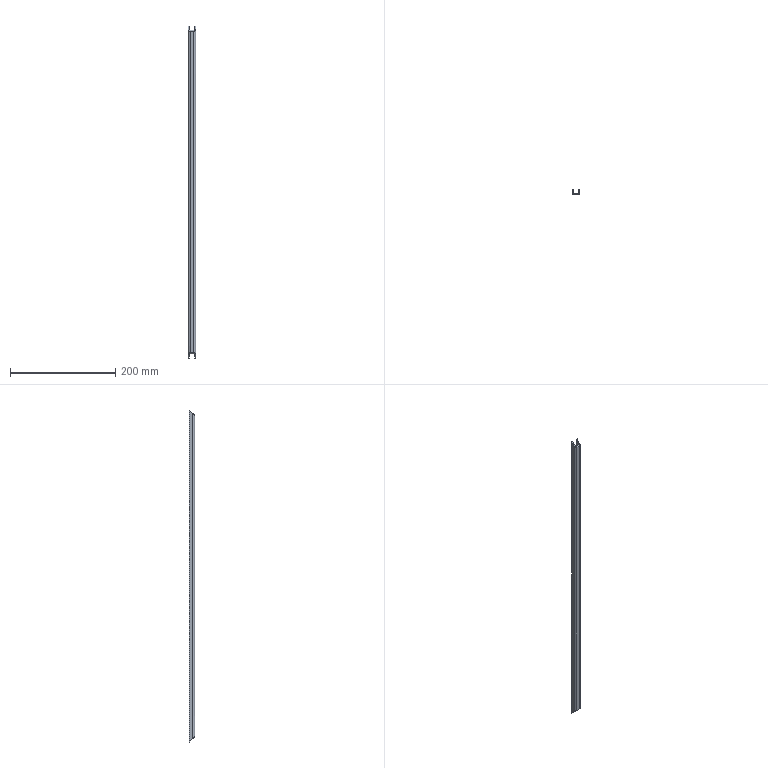Part | STEP file | 1 solid | 14 faces | box 14 x 10 x 632 mm | volume 34530 mm3 | plane 10 | cylinder 4 | commonest cylinder face diameters 3 x2 7 x2
STEP:
#1=CARTESIAN_POINT('',(0.,0.,0.));
#2=DIRECTION('',(0.,0.,1.));
#3=DIRECTION('',(1.,0.,0.));
#4=AXIS2_PLACEMENT_3D('',#1,#2,#3);
#5=CARTESIAN_POINT('',(-5.,5.,632.));
#6=VERTEX_POINT('',#5);
#7=CARTESIAN_POINT('',(-5.,5.,0.));
#8=VERTEX_POINT('',#7);
#9=CARTESIAN_POINT('',(-5.,5.,632.));
#10=DIRECTION('',(0.,0.,-1.));
#11=VECTOR('',#10,1.);
#12=LINE('',#9,#11);
#13=CARTESIAN_POINT('',(-5.,-5.,632.));
#14=DIRECTION('',(-1.,0.,0.));
#15=DIRECTION('',(0.,0.,1.));
#16=AXIS2_PLACEMENT_3D('',#13,#14,#15);
#17=PLANE('',#16);
#18=CARTESIAN_POINT('',(0.,10.));
#19=DIRECTION('',(-1.,0.));
#20=VECTOR('',#19,1.);
#21=LINE('',#18,#20);
#22=(GEOMETRIC_REPRESENTATION_CONTEXT(2)PARAMETRIC_REPRESENTATION_CONTEXT()REPRESENTATION_CONTEXT('',''));
#23=DEFINITIONAL_REPRESENTATION('',(#21),#22);
#24=PCURVE('',#17,#23);
#25=CARTESIAN_POINT('',(-7.,5.,632.));
#26=DIRECTION('',(0.,1.,0.));
#27=DIRECTION('',(0.,0.,1.));
#28=AXIS2_PLACEMENT_3D('',#25,#26,#27);
#29=PLANE('',#28);
#30=CARTESIAN_POINT('',(0.,2.));
#31=DIRECTION('',(-1.,0.));
#32=VECTOR('',#31,1.);
#33=LINE('',#30,#32);
#34=(GEOMETRIC_REPRESENTATION_CONTEXT(2)PARAMETRIC_REPRESENTATION_CONTEXT()REPRESENTATION_CONTEXT('',''));
#35=DEFINITIONAL_REPRESENTATION('',(#33),#34);
#36=PCURVE('',#29,#35);
#37=SURFACE_CURVE('',#12,(#24,#36),.PCURVE_S1.);
#38=EDGE_CURVE('',#6,#8,#37,.T.);
#39=ORIENTED_EDGE('',*,*,#38,.F.);
#40=CARTESIAN_POINT('',(-5.,-1.5,625.5));
#41=VERTEX_POINT('',#40);
#42=CARTESIAN_POINT('',(-5.,0.,627.));
#43=DIRECTION('',(0.,-0.7071,-0.7071));
#44=VECTOR('',#43,1.);
#45=LINE('',#42,#44);
#46=CARTESIAN_POINT('',(-5.,5.));
#47=DIRECTION('',(-0.7071,-0.7071));
#48=VECTOR('',#47,1.);
#49=LINE('',#46,#48);
#50=(GEOMETRIC_REPRESENTATION_CONTEXT(2)PARAMETRIC_REPRESENTATION_CONTEXT()REPRESENTATION_CONTEXT('',''));
#51=DEFINITIONAL_REPRESENTATION('',(#49),#50);
#52=PCURVE('',#17,#51);
#53=CARTESIAN_POINT('',(-63.,5.,632.));
#54=DIRECTION('',(0.,0.7071,-0.7071));
#55=DIRECTION('',(0.,0.7071,0.7071));
#56=AXIS2_PLACEMENT_3D('',#53,#54,#55);
#57=PLANE('',#56);
#58=CARTESIAN_POINT('',(-7.071,58.));
#59=DIRECTION('',(-1.,0.));
#60=VECTOR('',#59,1.);
#61=LINE('',#58,#60);
#62=(GEOMETRIC_REPRESENTATION_CONTEXT(2)PARAMETRIC_REPRESENTATION_CONTEXT()REPRESENTATION_CONTEXT('',''));
#63=DEFINITIONAL_REPRESENTATION('',(#61),#62);
#64=PCURVE('',#57,#63);
#65=SURFACE_CURVE('',#45,(#52,#64),.PCURVE_S1.);
#66=EDGE_CURVE('',#6,#41,#65,.T.);
#67=ORIENTED_EDGE('',*,*,#66,.T.);
#68=CARTESIAN_POINT('',(-5.,-1.5,6.5));
#69=VERTEX_POINT('',#68);
#70=CARTESIAN_POINT('',(-5.,-1.5,632.));
#71=DIRECTION('',(0.,0.,-1.));
#72=VECTOR('',#71,1.);
#73=LINE('',#70,#72);
#74=CARTESIAN_POINT('',(0.,3.5));
#75=DIRECTION('',(-1.,0.));
#76=VECTOR('',#75,1.);
#77=LINE('',#74,#76);
#78=(GEOMETRIC_REPRESENTATION_CONTEXT(2)PARAMETRIC_REPRESENTATION_CONTEXT()REPRESENTATION_CONTEXT('',''));
#79=DEFINITIONAL_REPRESENTATION('',(#77),#78);
#80=PCURVE('',#17,#79);
#81=CARTESIAN_POINT('',(-3.5,-1.5,632.));
#82=DIRECTION('',(0.,0.,-1.));
#83=DIRECTION('',(-1.,0.,0.));
#84=AXIS2_PLACEMENT_3D('',#81,#82,#83);
#85=CYLINDRICAL_SURFACE('',#84,1.5);
#86=CARTESIAN_POINT('',(6.283,0.));
#87=DIRECTION('',(0.,1.));
#88=VECTOR('',#87,1.);
#89=LINE('',#86,#88);
#90=(GEOMETRIC_REPRESENTATION_CONTEXT(2)PARAMETRIC_REPRESENTATION_CONTEXT()REPRESENTATION_CONTEXT('',''));
#91=DEFINITIONAL_REPRESENTATION('',(#89),#90);
#92=PCURVE('',#85,#91);
#93=SURFACE_CURVE('',#73,(#80,#92),.PCURVE_S1.);
#94=EDGE_CURVE('',#41,#69,#93,.T.);
#95=ORIENTED_EDGE('',*,*,#94,.T.);
#96=CARTESIAN_POINT('',(-5.,-316.,321.));
#97=DIRECTION('',(0.,0.7071,-0.7071));
#98=VECTOR('',#97,1.);
#99=LINE('',#96,#98);
#100=CARTESIAN_POINT('',(-311.,-311.));
#101=DIRECTION('',(-0.7071,0.7071));
#102=VECTOR('',#101,1.);
#103=LINE('',#100,#102);
#104=(GEOMETRIC_REPRESENTATION_CONTEXT(2)PARAMETRIC_REPRESENTATION_CONTEXT()REPRESENTATION_CONTEXT('',''));
#105=DEFINITIONAL_REPRESENTATION('',(#103),#104);
#106=PCURVE('',#17,#105);
#107=CARTESIAN_POINT('',(-63.,5.,0.));
#108=DIRECTION('',(0.,0.7071,0.7071));
#109=DIRECTION('',(0.,-0.7071,0.7071));
#110=AXIS2_PLACEMENT_3D('',#107,#108,#109);
#111=PLANE('',#110);
#112=CARTESIAN_POINT('',(453.963,58.));
#113=DIRECTION('',(-1.,0.));
#114=VECTOR('',#113,1.);
#115=LINE('',#112,#114);
#116=(GEOMETRIC_REPRESENTATION_CONTEXT(2)PARAMETRIC_REPRESENTATION_CONTEXT()REPRESENTATION_CONTEXT('',''));
#117=DEFINITIONAL_REPRESENTATION('',(#115),#116);
#118=PCURVE('',#111,#117);
#119=SURFACE_CURVE('',#99,(#106,#118),.PCURVE_S1.);
#120=EDGE_CURVE('',#69,#8,#119,.T.);
#121=ORIENTED_EDGE('',*,*,#120,.T.);
#122=EDGE_LOOP('',(#39,#67,#95,#121));
#123=FACE_BOUND('',#122,.T.);
#124=ADVANCED_FACE('',(#123),#17,.F.);
#125=CARTESIAN_POINT('',(-7.,5.,0.));
#126=VERTEX_POINT('',#125);
#127=CARTESIAN_POINT('',(-7.,5.,0.));
#128=DIRECTION('',(1.,0.,0.));
#129=VECTOR('',#128,1.);
#130=LINE('',#127,#129);
#131=CARTESIAN_POINT('',(-632.,0.));
#132=DIRECTION('',(0.,1.));
#133=VECTOR('',#132,1.);
#134=LINE('',#131,#133);
#135=(GEOMETRIC_REPRESENTATION_CONTEXT(2)PARAMETRIC_REPRESENTATION_CONTEXT()REPRESENTATION_CONTEXT('',''));
#136=DEFINITIONAL_REPRESENTATION('',(#134),#135);
#137=PCURVE('',#29,#136);
#138=CARTESIAN_POINT('',(0.,56.));
#139=DIRECTION('',(0.,1.));
#140=VECTOR('',#139,1.);
#141=LINE('',#138,#140);
#142=(GEOMETRIC_REPRESENTATION_CONTEXT(2)PARAMETRIC_REPRESENTATION_CONTEXT()REPRESENTATION_CONTEXT('',''));
#143=DEFINITIONAL_REPRESENTATION('',(#141),#142);
#144=PCURVE('',#111,#143);
#145=SURFACE_CURVE('',#130,(#137,#144),.PCURVE_S1.);
#146=EDGE_CURVE('',#126,#8,#145,.T.);
#147=ORIENTED_EDGE('',*,*,#146,.F.);
#148=CARTESIAN_POINT('',(-7.,5.,632.));
#149=VERTEX_POINT('',#148);
#150=CARTESIAN_POINT('',(-7.,5.,632.));
#151=DIRECTION('',(0.,0.,-1.));
#152=VECTOR('',#151,1.);
#153=LINE('',#150,#152);
#154=CARTESIAN_POINT('',(0.,0.));
#155=DIRECTION('',(-1.,0.));
#156=VECTOR('',#155,1.);
#157=LINE('',#154,#156);
#158=(GEOMETRIC_REPRESENTATION_CONTEXT(2)PARAMETRIC_REPRESENTATION_CONTEXT()REPRESENTATION_CONTEXT('',''));
#159=DEFINITIONAL_REPRESENTATION('',(#157),#158);
#160=PCURVE('',#29,#159);
#161=CARTESIAN_POINT('',(-7.,-5.,632.));
#162=DIRECTION('',(-1.,0.,0.));
#163=DIRECTION('',(0.,0.,1.));
#164=AXIS2_PLACEMENT_3D('',#161,#162,#163);
#165=PLANE('',#164);
#166=CARTESIAN_POINT('',(0.,10.));
#167=DIRECTION('',(-1.,0.));
#168=VECTOR('',#167,1.);
#169=LINE('',#166,#168);
#170=(GEOMETRIC_REPRESENTATION_CONTEXT(2)PARAMETRIC_REPRESENTATION_CONTEXT()REPRESENTATION_CONTEXT('',''));
#171=DEFINITIONAL_REPRESENTATION('',(#169),#170);
#172=PCURVE('',#165,#171);
#173=SURFACE_CURVE('',#153,(#160,#172),.PCURVE_S1.);
#174=EDGE_CURVE('',#149,#126,#173,.T.);
#175=ORIENTED_EDGE('',*,*,#174,.F.);
#176=CARTESIAN_POINT('',(-7.,5.,632.));
#177=DIRECTION('',(1.,0.,0.));
#178=VECTOR('',#177,1.);
#179=LINE('',#176,#178);
#180=CARTESIAN_POINT('',(0.,0.));
#181=DIRECTION('',(0.,1.));
#182=VECTOR('',#181,1.);
#183=LINE('',#180,#182);
#184=(GEOMETRIC_REPRESENTATION_CONTEXT(2)PARAMETRIC_REPRESENTATION_CONTEXT()REPRESENTATION_CONTEXT('',''));
#185=DEFINITIONAL_REPRESENTATION('',(#183),#184);
#186=PCURVE('',#29,#185);
#187=CARTESIAN_POINT('',(0.,56.));
#188=DIRECTION('',(0.,1.));
#189=VECTOR('',#188,1.);
#190=LINE('',#187,#189);
#191=(GEOMETRIC_REPRESENTATION_CONTEXT(2)PARAMETRIC_REPRESENTATION_CONTEXT()REPRESENTATION_CONTEXT('',''));
#192=DEFINITIONAL_REPRESENTATION('',(#190),#191);
#193=PCURVE('',#57,#192);
#194=SURFACE_CURVE('',#179,(#186,#193),.PCURVE_S1.);
#195=EDGE_CURVE('',#149,#6,#194,.T.);
#196=ORIENTED_EDGE('',*,*,#195,.T.);
#197=ORIENTED_EDGE('',*,*,#38,.T.);
#198=EDGE_LOOP('',(#147,#175,#196,#197));
#199=FACE_BOUND('',#198,.T.);
#200=ADVANCED_FACE('',(#199),#29,.T.);
#201=CARTESIAN_POINT('',(-7.,-1.5,625.5));
#202=VERTEX_POINT('',#201);
#203=CARTESIAN_POINT('',(-7.,0.,627.));
#204=DIRECTION('',(0.,-0.7071,-0.7071));
#205=VECTOR('',#204,1.);
#206=LINE('',#203,#205);
#207=CARTESIAN_POINT('',(-5.,5.));
#208=DIRECTION('',(-0.7071,-0.7071));
#209=VECTOR('',#208,1.);
#210=LINE('',#207,#209);
#211=(GEOMETRIC_REPRESENTATION_CONTEXT(2)PARAMETRIC_REPRESENTATION_CONTEXT()REPRESENTATION_CONTEXT('',''));
#212=DEFINITIONAL_REPRESENTATION('',(#210),#211);
#213=PCURVE('',#165,#212);
#214=CARTESIAN_POINT('',(-7.071,56.));
#215=DIRECTION('',(-1.,0.));
#216=VECTOR('',#215,1.);
#217=LINE('',#214,#216);
#218=(GEOMETRIC_REPRESENTATION_CONTEXT(2)PARAMETRIC_REPRESENTATION_CONTEXT()REPRESENTATION_CONTEXT('',''));
#219=DEFINITIONAL_REPRESENTATION('',(#217),#218);
#220=PCURVE('',#57,#219);
#221=SURFACE_CURVE('',#206,(#213,#220),.PCURVE_S1.);
#222=EDGE_CURVE('',#149,#202,#221,.T.);
#223=ORIENTED_EDGE('',*,*,#222,.F.);
#224=ORIENTED_EDGE('',*,*,#174,.T.);
#225=CARTESIAN_POINT('',(-7.,-1.5,6.5));
#226=VERTEX_POINT('',#225);
#227=CARTESIAN_POINT('',(-7.,-316.,321.));
#228=DIRECTION('',(0.,0.7071,-0.7071));
#229=VECTOR('',#228,1.);
#230=LINE('',#227,#229);
#231=CARTESIAN_POINT('',(-311.,-311.));
#232=DIRECTION('',(-0.7071,0.7071));
#233=VECTOR('',#232,1.);
#234=LINE('',#231,#233);
#235=(GEOMETRIC_REPRESENTATION_CONTEXT(2)PARAMETRIC_REPRESENTATION_CONTEXT()REPRESENTATION_CONTEXT('',''));
#236=DEFINITIONAL_REPRESENTATION('',(#234),#235);
#237=PCURVE('',#165,#236);
#238=CARTESIAN_POINT('',(453.963,56.));
#239=DIRECTION('',(-1.,0.));
#240=VECTOR('',#239,1.);
#241=LINE('',#238,#240);
#242=(GEOMETRIC_REPRESENTATION_CONTEXT(2)PARAMETRIC_REPRESENTATION_CONTEXT()REPRESENTATION_CONTEXT('',''));
#243=DEFINITIONAL_REPRESENTATION('',(#241),#242);
#244=PCURVE('',#111,#243);
#245=SURFACE_CURVE('',#230,(#237,#244),.PCURVE_S1.);
#246=EDGE_CURVE('',#226,#126,#245,.T.);
#247=ORIENTED_EDGE('',*,*,#246,.F.);
#248=CARTESIAN_POINT('',(-7.,-1.5,632.));
#249=DIRECTION('',(0.,0.,-1.));
#250=VECTOR('',#249,1.);
#251=LINE('',#248,#250);
#252=CARTESIAN_POINT('',(0.,3.5));
#253=DIRECTION('',(-1.,0.));
#254=VECTOR('',#253,1.);
#255=LINE('',#252,#254);
#256=(GEOMETRIC_REPRESENTATION_CONTEXT(2)PARAMETRIC_REPRESENTATION_CONTEXT()REPRESENTATION_CONTEXT('',''));
#257=DEFINITIONAL_REPRESENTATION('',(#255),#256);
#258=PCURVE('',#165,#257);
#259=CARTESIAN_POINT('',(-3.5,-1.5,632.));
#260=DIRECTION('',(0.,0.,-1.));
#261=DIRECTION('',(-1.,0.,0.));
#262=AXIS2_PLACEMENT_3D('',#259,#260,#261);
#263=CYLINDRICAL_SURFACE('',#262,3.5);
#264=CARTESIAN_POINT('',(6.283,0.));
#265=DIRECTION('',(0.,1.));
#266=VECTOR('',#265,1.);
#267=LINE('',#264,#266);
#268=(GEOMETRIC_REPRESENTATION_CONTEXT(2)PARAMETRIC_REPRESENTATION_CONTEXT()REPRESENTATION_CONTEXT('',''));
#269=DEFINITIONAL_REPRESENTATION('',(#267),#268);
#270=PCURVE('',#263,#269);
#271=SURFACE_CURVE('',#251,(#258,#270),.PCURVE_S1.);
#272=EDGE_CURVE('',#202,#226,#271,.T.);
#273=ORIENTED_EDGE('',*,*,#272,.F.);
#274=EDGE_LOOP('',(#223,#224,#247,#273));
#275=FACE_BOUND('',#274,.T.);
#276=ADVANCED_FACE('',(#275),#165,.T.);
#277=CARTESIAN_POINT('',(-3.5,-5.,622.));
#278=VERTEX_POINT('',#277);
#279=CARTESIAN_POINT('',(-7.,-1.5,625.5));
#280=CARTESIAN_POINT('',(-7.,-3.55,623.45));
#281=CARTESIAN_POINT('',(-5.55,-5.,622.));
#282=CARTESIAN_POINT('',(-3.5,-5.,622.));
#283=(BOUNDED_CURVE()B_SPLINE_CURVE(3,(#279,#280,#281,#282),.UNSPECIFIED.,.F.,.F.)B_SPLINE_CURVE_WITH_KNOTS((4,4),(4.712,6.283),.PIECEWISE_BEZIER_KNOTS.)CURVE()GEOMETRIC_REPRESENTATION_ITEM()RATIONAL_B_SPLINE_CURVE((1.,0.8047,0.8047,1.))REPRESENTATION_ITEM(''));
#284=CARTESIAN_POINT('',(6.283,6.5));
#285=CARTESIAN_POINT('',(6.262,6.575));
#286=CARTESIAN_POINT('',(6.218,6.727));
#287=CARTESIAN_POINT('',(6.152,6.96));
#288=CARTESIAN_POINT('',(6.083,7.196));
#289=CARTESIAN_POINT('',(6.013,7.433));
#290=CARTESIAN_POINT('',(5.942,7.671));
#291=CARTESIAN_POINT('',(5.87,7.906));
#292=CARTESIAN_POINT('',(5.797,8.137));
#293=CARTESIAN_POINT('',(5.723,8.362));
#294=CARTESIAN_POINT('',(5.648,8.578));
#295=CARTESIAN_POINT('',(5.573,8.784));
#296=CARTESIAN_POINT('',(5.498,8.977));
#297=CARTESIAN_POINT('',(5.422,9.157));
#298=CARTESIAN_POINT('',(5.347,9.32));
#299=CARTESIAN_POINT('',(5.273,9.468));
#300=CARTESIAN_POINT('',(5.199,9.597));
#301=CARTESIAN_POINT('',(5.125,9.709));
#302=CARTESIAN_POINT('',(5.053,9.802));
#303=CARTESIAN_POINT('',(4.982,9.876));
#304=CARTESIAN_POINT('',(4.912,9.933));
#305=CARTESIAN_POINT('',(4.844,9.972));
#306=CARTESIAN_POINT('',(4.777,9.995));
#307=CARTESIAN_POINT('',(4.734,10.));
#308=CARTESIAN_POINT('',(4.712,10.));
#309=B_SPLINE_CURVE_WITH_KNOTS('',3,(#284,#285,#286,#287,#288,#289,#290,#291,#292,#293,#294,#295,#296,#297,#298,#299,#300,#301,#302,#303,#304,#305,#306,#307,#308),.UNSPECIFIED.,.F.,.F.,(4,1,1,1,1,1,1,1,1,1,1,1,1,1,1,1,1,1,1,1,1,1,4),(4.712,4.784,4.855,4.927,4.998,5.069,5.141,5.212,5.284,5.355,5.426,5.498,5.569,5.641,5.712,5.783,5.855,5.926,5.998,6.069,6.14,6.212,6.283),.QUASI_UNIFORM_KNOTS.);
#310=(GEOMETRIC_REPRESENTATION_CONTEXT(2)PARAMETRIC_REPRESENTATION_CONTEXT()REPRESENTATION_CONTEXT('',''));
#311=DEFINITIONAL_REPRESENTATION('',(#309),#310);
#312=PCURVE('',#263,#311);
#313=CARTESIAN_POINT('',(-9.192,56.));
#314=CARTESIAN_POINT('',(-12.092,56.));
#315=CARTESIAN_POINT('',(-14.142,57.45));
#316=CARTESIAN_POINT('',(-14.142,59.5));
#317=(BOUNDED_CURVE()B_SPLINE_CURVE(3,(#313,#314,#315,#316),.UNSPECIFIED.,.F.,.F.)B_SPLINE_CURVE_WITH_KNOTS((4,4),(4.712,6.283),.PIECEWISE_BEZIER_KNOTS.)CURVE()GEOMETRIC_REPRESENTATION_ITEM()RATIONAL_B_SPLINE_CURVE((1.,0.8047,0.8047,1.))REPRESENTATION_ITEM(''));
#318=(GEOMETRIC_REPRESENTATION_CONTEXT(2)PARAMETRIC_REPRESENTATION_CONTEXT()REPRESENTATION_CONTEXT('',''));
#319=DEFINITIONAL_REPRESENTATION('',(#317),#318);
#320=PCURVE('',#57,#319);
#321=SURFACE_CURVE('',#283,(#312,#320),.PCURVE_S1.);
#322=EDGE_CURVE('',#202,#278,#321,.T.);
#323=ORIENTED_EDGE('',*,*,#322,.F.);
#324=ORIENTED_EDGE('',*,*,#272,.T.);
#325=CARTESIAN_POINT('',(-3.5,-5.,10.));
#326=VERTEX_POINT('',#325);
#327=CARTESIAN_POINT('',(-3.5,-5.,10.));
#328=CARTESIAN_POINT('',(-5.55,-5.,10.));
#329=CARTESIAN_POINT('',(-7.,-3.55,8.55));
#330=CARTESIAN_POINT('',(-7.,-1.5,6.5));
#331=(BOUNDED_CURVE()B_SPLINE_CURVE(3,(#327,#328,#329,#330),.UNSPECIFIED.,.F.,.F.)B_SPLINE_CURVE_WITH_KNOTS((4,4),(3.142,4.712),.PIECEWISE_BEZIER_KNOTS.)CURVE()GEOMETRIC_REPRESENTATION_ITEM()RATIONAL_B_SPLINE_CURVE((1.,0.8047,0.8047,1.))REPRESENTATION_ITEM(''));
#332=CARTESIAN_POINT('',(4.712,622.));
#333=CARTESIAN_POINT('',(4.734,622.));
#334=CARTESIAN_POINT('',(4.777,622.005));
#335=CARTESIAN_POINT('',(4.844,622.028));
#336=CARTESIAN_POINT('',(4.912,622.067));
#337=CARTESIAN_POINT('',(4.982,622.124));
#338=CARTESIAN_POINT('',(5.053,622.198));
#339=CARTESIAN_POINT('',(5.125,622.291));
#340=CARTESIAN_POINT('',(5.199,622.403));
#341=CARTESIAN_POINT('',(5.273,622.532));
#342=CARTESIAN_POINT('',(5.347,622.68));
#343=CARTESIAN_POINT('',(5.422,622.843));
#344=CARTESIAN_POINT('',(5.498,623.023));
#345=CARTESIAN_POINT('',(5.573,623.216));
#346=CARTESIAN_POINT('',(5.648,623.422));
#347=CARTESIAN_POINT('',(5.723,623.638));
#348=CARTESIAN_POINT('',(5.797,623.863));
#349=CARTESIAN_POINT('',(5.87,624.094));
#350=CARTESIAN_POINT('',(5.942,624.329));
#351=CARTESIAN_POINT('',(6.013,624.567));
#352=CARTESIAN_POINT('',(6.083,624.804));
#353=CARTESIAN_POINT('',(6.152,625.04));
#354=CARTESIAN_POINT('',(6.218,625.273));
#355=CARTESIAN_POINT('',(6.262,625.425));
#356=CARTESIAN_POINT('',(6.283,625.5));
#357=B_SPLINE_CURVE_WITH_KNOTS('',3,(#332,#333,#334,#335,#336,#337,#338,#339,#340,#341,#342,#343,#344,#345,#346,#347,#348,#349,#350,#351,#352,#353,#354,#355,#356),.UNSPECIFIED.,.F.,.F.,(4,1,1,1,1,1,1,1,1,1,1,1,1,1,1,1,1,1,1,1,1,1,4),(3.142,3.213,3.284,3.356,3.427,3.499,3.57,3.641,3.713,3.784,3.856,3.927,3.998,4.07,4.141,4.213,4.284,4.355,4.427,4.498,4.57,4.641,4.712),.QUASI_UNIFORM_KNOTS.);
#358=(GEOMETRIC_REPRESENTATION_CONTEXT(2)PARAMETRIC_REPRESENTATION_CONTEXT()REPRESENTATION_CONTEXT('',''));
#359=DEFINITIONAL_REPRESENTATION('',(#357),#358);
#360=PCURVE('',#263,#359);
#361=CARTESIAN_POINT('',(14.142,59.5));
#362=CARTESIAN_POINT('',(14.142,57.45));
#363=CARTESIAN_POINT('',(12.092,56.));
#364=CARTESIAN_POINT('',(9.192,56.));
#365=(BOUNDED_CURVE()B_SPLINE_CURVE(3,(#361,#362,#363,#364),.UNSPECIFIED.,.F.,.F.)B_SPLINE_CURVE_WITH_KNOTS((4,4),(3.142,4.712),.PIECEWISE_BEZIER_KNOTS.)CURVE()GEOMETRIC_REPRESENTATION_ITEM()RATIONAL_B_SPLINE_CURVE((1.,0.8047,0.8047,1.))REPRESENTATION_ITEM(''));
#366=(GEOMETRIC_REPRESENTATION_CONTEXT(2)PARAMETRIC_REPRESENTATION_CONTEXT()REPRESENTATION_CONTEXT('',''));
#367=DEFINITIONAL_REPRESENTATION('',(#365),#366);
#368=PCURVE('',#111,#367);
#369=SURFACE_CURVE('',#331,(#360,#368),.PCURVE_S1.);
#370=EDGE_CURVE('',#326,#226,#369,.T.);
#371=ORIENTED_EDGE('',*,*,#370,.F.);
#372=CARTESIAN_POINT('',(-3.5,-5.,632.));
#373=DIRECTION('',(0.,0.,-1.));
#374=VECTOR('',#373,1.);
#375=LINE('',#372,#374);
#376=CARTESIAN_POINT('',(4.712,0.));
#377=DIRECTION('',(0.,1.));
#378=VECTOR('',#377,1.);
#379=LINE('',#376,#378);
#380=(GEOMETRIC_REPRESENTATION_CONTEXT(2)PARAMETRIC_REPRESENTATION_CONTEXT()REPRESENTATION_CONTEXT('',''));
#381=DEFINITIONAL_REPRESENTATION('',(#379),#380);
#382=PCURVE('',#263,#381);
#383=CARTESIAN_POINT('',(-7.,-5.,632.));
#384=DIRECTION('',(0.,-1.,0.));
#385=DIRECTION('',(0.,0.,-1.));
#386=AXIS2_PLACEMENT_3D('',#383,#384,#385);
#387=PLANE('',#386);
#388=CARTESIAN_POINT('',(0.,3.5));
#389=DIRECTION('',(1.,0.));
#390=VECTOR('',#389,1.);
#391=LINE('',#388,#390);
#392=(GEOMETRIC_REPRESENTATION_CONTEXT(2)PARAMETRIC_REPRESENTATION_CONTEXT()REPRESENTATION_CONTEXT('',''));
#393=DEFINITIONAL_REPRESENTATION('',(#391),#392);
#394=PCURVE('',#387,#393);
#395=SURFACE_CURVE('',#375,(#382,#394),.PCURVE_S1.);
#396=EDGE_CURVE('',#278,#326,#395,.T.);
#397=ORIENTED_EDGE('',*,*,#396,.F.);
#398=EDGE_LOOP('',(#323,#324,#371,#397));
#399=FACE_BOUND('',#398,.T.);
#400=ADVANCED_FACE('',(#399),#263,.T.);
#401=CARTESIAN_POINT('',(3.5,-5.,622.));
#402=VERTEX_POINT('',#401);
#403=CARTESIAN_POINT('',(-63.,-5.,622.));
#404=DIRECTION('',(1.,0.,0.));
#405=VECTOR('',#404,1.);
#406=LINE('',#403,#405);
#407=CARTESIAN_POINT('',(10.,-56.));
#408=DIRECTION('',(0.,1.));
#409=VECTOR('',#408,1.);
#410=LINE('',#407,#409);
#411=(GEOMETRIC_REPRESENTATION_CONTEXT(2)PARAMETRIC_REPRESENTATION_CONTEXT()REPRESENTATION_CONTEXT('',''));
#412=DEFINITIONAL_REPRESENTATION('',(#410),#411);
#413=PCURVE('',#387,#412);
#414=CARTESIAN_POINT('',(-14.142,0.));
#415=DIRECTION('',(0.,1.));
#416=VECTOR('',#415,1.);
#417=LINE('',#414,#416);
#418=(GEOMETRIC_REPRESENTATION_CONTEXT(2)PARAMETRIC_REPRESENTATION_CONTEXT()REPRESENTATION_CONTEXT('',''));
#419=DEFINITIONAL_REPRESENTATION('',(#417),#418);
#420=PCURVE('',#57,#419);
#421=SURFACE_CURVE('',#406,(#413,#420),.PCURVE_S1.);
#422=EDGE_CURVE('',#278,#402,#421,.T.);
#423=ORIENTED_EDGE('',*,*,#422,.F.);
#424=ORIENTED_EDGE('',*,*,#396,.T.);
#425=CARTESIAN_POINT('',(3.5,-5.,10.));
#426=VERTEX_POINT('',#425);
#427=CARTESIAN_POINT('',(-63.,-5.,10.));
#428=DIRECTION('',(1.,0.,0.));
#429=VECTOR('',#428,1.);
#430=LINE('',#427,#429);
#431=CARTESIAN_POINT('',(622.,-56.));
#432=DIRECTION('',(0.,1.));
#433=VECTOR('',#432,1.);
#434=LINE('',#431,#433);
#435=(GEOMETRIC_REPRESENTATION_CONTEXT(2)PARAMETRIC_REPRESENTATION_CONTEXT()REPRESENTATION_CONTEXT('',''));
#436=DEFINITIONAL_REPRESENTATION('',(#434),#435);
#437=PCURVE('',#387,#436);
#438=CARTESIAN_POINT('',(14.142,0.));
#439=DIRECTION('',(0.,1.));
#440=VECTOR('',#439,1.);
#441=LINE('',#438,#440);
#442=(GEOMETRIC_REPRESENTATION_CONTEXT(2)PARAMETRIC_REPRESENTATION_CONTEXT()REPRESENTATION_CONTEXT('',''));
#443=DEFINITIONAL_REPRESENTATION('',(#441),#442);
#444=PCURVE('',#111,#443);
#445=SURFACE_CURVE('',#430,(#437,#444),.PCURVE_S1.);
#446=EDGE_CURVE('',#326,#426,#445,.T.);
#447=ORIENTED_EDGE('',*,*,#446,.T.);
#448=CARTESIAN_POINT('',(3.5,-5.,632.));
#449=DIRECTION('',(0.,0.,-1.));
#450=VECTOR('',#449,1.);
#451=LINE('',#448,#450);
#452=CARTESIAN_POINT('',(0.,10.5));
#453=DIRECTION('',(1.,0.));
#454=VECTOR('',#453,1.);
#455=LINE('',#452,#454);
#456=(GEOMETRIC_REPRESENTATION_CONTEXT(2)PARAMETRIC_REPRESENTATION_CONTEXT()REPRESENTATION_CONTEXT('',''));
#457=DEFINITIONAL_REPRESENTATION('',(#455),#456);
#458=PCURVE('',#387,#457);
#459=CARTESIAN_POINT('',(3.5,-1.5,632.));
#460=DIRECTION('',(0.,0.,-1.));
#461=DIRECTION('',(-1.,0.,0.));
#462=AXIS2_PLACEMENT_3D('',#459,#460,#461);
#463=CYLINDRICAL_SURFACE('',#462,3.5);
#464=CARTESIAN_POINT('',(4.712,0.));
#465=DIRECTION('',(0.,1.));
#466=VECTOR('',#465,1.);
#467=LINE('',#464,#466);
#468=(GEOMETRIC_REPRESENTATION_CONTEXT(2)PARAMETRIC_REPRESENTATION_CONTEXT()REPRESENTATION_CONTEXT('',''));
#469=DEFINITIONAL_REPRESENTATION('',(#467),#468);
#470=PCURVE('',#463,#469);
#471=SURFACE_CURVE('',#451,(#458,#470),.PCURVE_S1.);
#472=EDGE_CURVE('',#402,#426,#471,.T.);
#473=ORIENTED_EDGE('',*,*,#472,.F.);
#474=EDGE_LOOP('',(#423,#424,#447,#473));
#475=FACE_BOUND('',#474,.T.);
#476=ADVANCED_FACE('',(#475),#387,.T.);
#477=CARTESIAN_POINT('',(7.,-1.5,625.5));
#478=VERTEX_POINT('',#477);
#479=CARTESIAN_POINT('',(3.5,-5.,622.));
#480=CARTESIAN_POINT('',(5.55,-5.,622.));
#481=CARTESIAN_POINT('',(7.,-3.55,623.45));
#482=CARTESIAN_POINT('',(7.,-1.5,625.5));
#483=(BOUNDED_CURVE()B_SPLINE_CURVE(3,(#479,#480,#481,#482),.UNSPECIFIED.,.F.,.F.)B_SPLINE_CURVE_WITH_KNOTS((4,4),(0.,1.571),.PIECEWISE_BEZIER_KNOTS.)CURVE()GEOMETRIC_REPRESENTATION_ITEM()RATIONAL_B_SPLINE_CURVE((1.,0.8047,0.8047,1.))REPRESENTATION_ITEM(''));
#484=CARTESIAN_POINT('',(4.712,10.));
#485=CARTESIAN_POINT('',(4.691,10.));
#486=CARTESIAN_POINT('',(4.648,9.995));
#487=CARTESIAN_POINT('',(4.581,9.972));
#488=CARTESIAN_POINT('',(4.512,9.933));
#489=CARTESIAN_POINT('',(4.443,9.876));
#490=CARTESIAN_POINT('',(4.372,9.802));
#491=CARTESIAN_POINT('',(4.299,9.709));
#492=CARTESIAN_POINT('',(4.226,9.597));
#493=CARTESIAN_POINT('',(4.152,9.468));
#494=CARTESIAN_POINT('',(4.077,9.32));
#495=CARTESIAN_POINT('',(4.002,9.157));
#496=CARTESIAN_POINT('',(3.927,8.977));
#497=CARTESIAN_POINT('',(3.852,8.784));
#498=CARTESIAN_POINT('',(3.777,8.578));
#499=CARTESIAN_POINT('',(3.702,8.362));
#500=CARTESIAN_POINT('',(3.628,8.137));
#501=CARTESIAN_POINT('',(3.555,7.906));
#502=CARTESIAN_POINT('',(3.482,7.671));
#503=CARTESIAN_POINT('',(3.411,7.433));
#504=CARTESIAN_POINT('',(3.342,7.196));
#505=CARTESIAN_POINT('',(3.273,6.96));
#506=CARTESIAN_POINT('',(3.206,6.727));
#507=CARTESIAN_POINT('',(3.163,6.575));
#508=CARTESIAN_POINT('',(3.142,6.5));
#509=B_SPLINE_CURVE_WITH_KNOTS('',3,(#484,#485,#486,#487,#488,#489,#490,#491,#492,#493,#494,#495,#496,#497,#498,#499,#500,#501,#502,#503,#504,#505,#506,#507,#508),.UNSPECIFIED.,.F.,.F.,(4,1,1,1,1,1,1,1,1,1,1,1,1,1,1,1,1,1,1,1,1,1,4),(0.,0.0714,0.1428,0.2142,0.2856,0.357,0.4284,0.4998,0.5712,0.6426,0.714,0.7854,0.8568,0.9282,0.9996,1.071,1.142,1.214,1.285,1.357,1.428,1.499,1.571),.QUASI_UNIFORM_KNOTS.);
#510=(GEOMETRIC_REPRESENTATION_CONTEXT(2)PARAMETRIC_REPRESENTATION_CONTEXT()REPRESENTATION_CONTEXT('',''));
#511=DEFINITIONAL_REPRESENTATION('',(#509),#510);
#512=PCURVE('',#463,#511);
#513=CARTESIAN_POINT('',(-14.142,66.5));
#514=CARTESIAN_POINT('',(-14.142,68.55));
#515=CARTESIAN_POINT('',(-12.092,70.));
#516=CARTESIAN_POINT('',(-9.192,70.));
#517=(BOUNDED_CURVE()B_SPLINE_CURVE(3,(#513,#514,#515,#516),.UNSPECIFIED.,.F.,.F.)B_SPLINE_CURVE_WITH_KNOTS((4,4),(0.,1.571),.PIECEWISE_BEZIER_KNOTS.)CURVE()GEOMETRIC_REPRESENTATION_ITEM()RATIONAL_B_SPLINE_CURVE((1.,0.8047,0.8047,1.))REPRESENTATION_ITEM(''));
#518=(GEOMETRIC_REPRESENTATION_CONTEXT(2)PARAMETRIC_REPRESENTATION_CONTEXT()REPRESENTATION_CONTEXT('',''));
#519=DEFINITIONAL_REPRESENTATION('',(#517),#518);
#520=PCURVE('',#57,#519);
#521=SURFACE_CURVE('',#483,(#512,#520),.PCURVE_S1.);
#522=EDGE_CURVE('',#402,#478,#521,.T.);
#523=ORIENTED_EDGE('',*,*,#522,.F.);
#524=ORIENTED_EDGE('',*,*,#472,.T.);
#525=CARTESIAN_POINT('',(7.,-1.5,6.5));
#526=VERTEX_POINT('',#525);
#527=CARTESIAN_POINT('',(7.,-1.5,6.5));
#528=CARTESIAN_POINT('',(7.,-3.55,8.55));
#529=CARTESIAN_POINT('',(5.55,-5.,10.));
#530=CARTESIAN_POINT('',(3.5,-5.,10.));
#531=(BOUNDED_CURVE()B_SPLINE_CURVE(3,(#527,#528,#529,#530),.UNSPECIFIED.,.F.,.F.)B_SPLINE_CURVE_WITH_KNOTS((4,4),(1.571,3.142),.PIECEWISE_BEZIER_KNOTS.)CURVE()GEOMETRIC_REPRESENTATION_ITEM()RATIONAL_B_SPLINE_CURVE((1.,0.8047,0.8047,1.))REPRESENTATION_ITEM(''));
#532=CARTESIAN_POINT('',(3.142,625.5));
#533=CARTESIAN_POINT('',(3.163,625.425));
#534=CARTESIAN_POINT('',(3.206,625.273));
#535=CARTESIAN_POINT('',(3.273,625.04));
#536=CARTESIAN_POINT('',(3.342,624.804));
#537=CARTESIAN_POINT('',(3.411,624.567));
#538=CARTESIAN_POINT('',(3.482,624.329));
#539=CARTESIAN_POINT('',(3.555,624.094));
#540=CARTESIAN_POINT('',(3.628,623.863));
#541=CARTESIAN_POINT('',(3.702,623.638));
#542=CARTESIAN_POINT('',(3.777,623.422));
#543=CARTESIAN_POINT('',(3.852,623.216));
#544=CARTESIAN_POINT('',(3.927,623.023));
#545=CARTESIAN_POINT('',(4.002,622.843));
#546=CARTESIAN_POINT('',(4.077,622.68));
#547=CARTESIAN_POINT('',(4.152,622.532));
#548=CARTESIAN_POINT('',(4.226,622.403));
#549=CARTESIAN_POINT('',(4.299,622.291));
#550=CARTESIAN_POINT('',(4.372,622.198));
#551=CARTESIAN_POINT('',(4.443,622.124));
#552=CARTESIAN_POINT('',(4.512,622.067));
#553=CARTESIAN_POINT('',(4.581,622.028));
#554=CARTESIAN_POINT('',(4.648,622.005));
#555=CARTESIAN_POINT('',(4.691,622.));
#556=CARTESIAN_POINT('',(4.712,622.));
#557=B_SPLINE_CURVE_WITH_KNOTS('',3,(#532,#533,#534,#535,#536,#537,#538,#539,#540,#541,#542,#543,#544,#545,#546,#547,#548,#549,#550,#551,#552,#553,#554,#555,#556),.UNSPECIFIED.,.F.,.F.,(4,1,1,1,1,1,1,1,1,1,1,1,1,1,1,1,1,1,1,1,1,1,4),(1.571,1.642,1.714,1.785,1.856,1.928,1.999,2.071,2.142,2.213,2.285,2.356,2.428,2.499,2.57,2.642,2.713,2.785,2.856,2.927,2.999,3.07,3.142),.QUASI_UNIFORM_KNOTS.);
#558=(GEOMETRIC_REPRESENTATION_CONTEXT(2)PARAMETRIC_REPRESENTATION_CONTEXT()REPRESENTATION_CONTEXT('',''));
#559=DEFINITIONAL_REPRESENTATION('',(#557),#558);
#560=PCURVE('',#463,#559);
#561=CARTESIAN_POINT('',(9.192,70.));
#562=CARTESIAN_POINT('',(12.092,70.));
#563=CARTESIAN_POINT('',(14.142,68.55));
#564=CARTESIAN_POINT('',(14.142,66.5));
#565=(BOUNDED_CURVE()B_SPLINE_CURVE(3,(#561,#562,#563,#564),.UNSPECIFIED.,.F.,.F.)B_SPLINE_CURVE_WITH_KNOTS((4,4),(1.571,3.142),.PIECEWISE_BEZIER_KNOTS.)CURVE()GEOMETRIC_REPRESENTATION_ITEM()RATIONAL_B_SPLINE_CURVE((1.,0.8047,0.8047,1.))REPRESENTATION_ITEM(''));
#566=(GEOMETRIC_REPRESENTATION_CONTEXT(2)PARAMETRIC_REPRESENTATION_CONTEXT()REPRESENTATION_CONTEXT('',''));
#567=DEFINITIONAL_REPRESENTATION('',(#565),#566);
#568=PCURVE('',#111,#567);
#569=SURFACE_CURVE('',#531,(#560,#568),.PCURVE_S1.);
#570=EDGE_CURVE('',#526,#426,#569,.T.);
#571=ORIENTED_EDGE('',*,*,#570,.F.);
#572=CARTESIAN_POINT('',(7.,-1.5,632.));
#573=DIRECTION('',(0.,0.,-1.));
#574=VECTOR('',#573,1.);
#575=LINE('',#572,#574);
#576=CARTESIAN_POINT('',(3.142,0.));
#577=DIRECTION('',(0.,1.));
#578=VECTOR('',#577,1.);
#579=LINE('',#576,#578);
#580=(GEOMETRIC_REPRESENTATION_CONTEXT(2)PARAMETRIC_REPRESENTATION_CONTEXT()REPRESENTATION_CONTEXT('',''));
#581=DEFINITIONAL_REPRESENTATION('',(#579),#580);
#582=PCURVE('',#463,#581);
#583=CARTESIAN_POINT('',(7.,-5.,632.));
#584=DIRECTION('',(1.,0.,0.));
#585=DIRECTION('',(0.,0.,-1.));
#586=AXIS2_PLACEMENT_3D('',#583,#584,#585);
#587=PLANE('',#586);
#588=CARTESIAN_POINT('',(0.,3.5));
#589=DIRECTION('',(1.,0.));
#590=VECTOR('',#589,1.);
#591=LINE('',#588,#590);
#592=(GEOMETRIC_REPRESENTATION_CONTEXT(2)PARAMETRIC_REPRESENTATION_CONTEXT()REPRESENTATION_CONTEXT('',''));
#593=DEFINITIONAL_REPRESENTATION('',(#591),#592);
#594=PCURVE('',#587,#593);
#595=SURFACE_CURVE('',#575,(#582,#594),.PCURVE_S1.);
#596=EDGE_CURVE('',#478,#526,#595,.T.);
#597=ORIENTED_EDGE('',*,*,#596,.F.);
#598=EDGE_LOOP('',(#523,#524,#571,#597));
#599=FACE_BOUND('',#598,.T.);
#600=ADVANCED_FACE('',(#599),#463,.T.);
#601=CARTESIAN_POINT('',(7.,5.,632.));
#602=VERTEX_POINT('',#601);
#603=CARTESIAN_POINT('',(7.,5.,632.));
#604=DIRECTION('',(0.,0.7071,0.7071));
#605=VECTOR('',#604,1.);
#606=LINE('',#603,#605);
#607=CARTESIAN_POINT('',(0.,10.));
#608=DIRECTION('',(-0.7071,0.7071));
#609=VECTOR('',#608,1.);
#610=LINE('',#607,#609);
#611=(GEOMETRIC_REPRESENTATION_CONTEXT(2)PARAMETRIC_REPRESENTATION_CONTEXT()REPRESENTATION_CONTEXT('',''));
#612=DEFINITIONAL_REPRESENTATION('',(#610),#611);
#613=PCURVE('',#587,#612);
#614=CARTESIAN_POINT('',(0.,70.));
#615=DIRECTION('',(1.,0.));
#616=VECTOR('',#615,1.);
#617=LINE('',#614,#616);
#618=(GEOMETRIC_REPRESENTATION_CONTEXT(2)PARAMETRIC_REPRESENTATION_CONTEXT()REPRESENTATION_CONTEXT('',''));
#619=DEFINITIONAL_REPRESENTATION('',(#617),#618);
#620=PCURVE('',#57,#619);
#621=SURFACE_CURVE('',#606,(#613,#620),.PCURVE_S1.);
#622=EDGE_CURVE('',#478,#602,#621,.T.);
#623=ORIENTED_EDGE('',*,*,#622,.F.);
#624=ORIENTED_EDGE('',*,*,#596,.T.);
#625=CARTESIAN_POINT('',(7.,5.,0.));
#626=VERTEX_POINT('',#625);
#627=CARTESIAN_POINT('',(7.,5.,0.));
#628=DIRECTION('',(0.,-0.7071,0.7071));
#629=VECTOR('',#628,1.);
#630=LINE('',#627,#629);
#631=CARTESIAN_POINT('',(632.,10.));
#632=DIRECTION('',(-0.7071,-0.7071));
#633=VECTOR('',#632,1.);
#634=LINE('',#631,#633);
#635=(GEOMETRIC_REPRESENTATION_CONTEXT(2)PARAMETRIC_REPRESENTATION_CONTEXT()REPRESENTATION_CONTEXT('',''));
#636=DEFINITIONAL_REPRESENTATION('',(#634),#635);
#637=PCURVE('',#587,#636);
#638=CARTESIAN_POINT('',(0.,70.));
#639=DIRECTION('',(1.,0.));
#640=VECTOR('',#639,1.);
#641=LINE('',#638,#640);
#642=(GEOMETRIC_REPRESENTATION_CONTEXT(2)PARAMETRIC_REPRESENTATION_CONTEXT()REPRESENTATION_CONTEXT('',''));
#643=DEFINITIONAL_REPRESENTATION('',(#641),#642);
#644=PCURVE('',#111,#643);
#645=SURFACE_CURVE('',#630,(#637,#644),.PCURVE_S1.);
#646=EDGE_CURVE('',#626,#526,#645,.T.);
#647=ORIENTED_EDGE('',*,*,#646,.F.);
#648=CARTESIAN_POINT('',(7.,5.,632.));
#649=DIRECTION('',(0.,0.,-1.));
#650=VECTOR('',#649,1.);
#651=LINE('',#648,#650);
#652=CARTESIAN_POINT('',(0.,10.));
#653=DIRECTION('',(1.,0.));
#654=VECTOR('',#653,1.);
#655=LINE('',#652,#654);
#656=(GEOMETRIC_REPRESENTATION_CONTEXT(2)PARAMETRIC_REPRESENTATION_CONTEXT()REPRESENTATION_CONTEXT('',''));
#657=DEFINITIONAL_REPRESENTATION('',(#655),#656);
#658=PCURVE('',#587,#657);
#659=CARTESIAN_POINT('',(5.,5.,632.));
#660=DIRECTION('',(0.,1.,0.));
#661=DIRECTION('',(0.,0.,1.));
#662=AXIS2_PLACEMENT_3D('',#659,#660,#661);
#663=PLANE('',#662);
#664=CARTESIAN_POINT('',(0.,2.));
#665=DIRECTION('',(-1.,0.));
#666=VECTOR('',#665,1.);
#667=LINE('',#664,#666);
#668=(GEOMETRIC_REPRESENTATION_CONTEXT(2)PARAMETRIC_REPRESENTATION_CONTEXT()REPRESENTATION_CONTEXT('',''));
#669=DEFINITIONAL_REPRESENTATION('',(#667),#668);
#670=PCURVE('',#663,#669);
#671=SURFACE_CURVE('',#651,(#658,#670),.PCURVE_S1.);
#672=EDGE_CURVE('',#602,#626,#671,.T.);
#673=ORIENTED_EDGE('',*,*,#672,.F.);
#674=EDGE_LOOP('',(#623,#624,#647,#673));
#675=FACE_BOUND('',#674,.T.);
#676=ADVANCED_FACE('',(#675),#587,.T.);
#677=CARTESIAN_POINT('',(5.,5.,0.));
#678=VERTEX_POINT('',#677);
#679=CARTESIAN_POINT('',(5.,5.,0.));
#680=DIRECTION('',(1.,0.,0.));
#681=VECTOR('',#680,1.);
#682=LINE('',#679,#681);
#683=CARTESIAN_POINT('',(-632.,0.));
#684=DIRECTION('',(0.,1.));
#685=VECTOR('',#684,1.);
#686=LINE('',#683,#685);
#687=(GEOMETRIC_REPRESENTATION_CONTEXT(2)PARAMETRIC_REPRESENTATION_CONTEXT()REPRESENTATION_CONTEXT('',''));
#688=DEFINITIONAL_REPRESENTATION('',(#686),#687);
#689=PCURVE('',#663,#688);
#690=CARTESIAN_POINT('',(0.,68.));
#691=DIRECTION('',(0.,1.));
#692=VECTOR('',#691,1.);
#693=LINE('',#690,#692);
#694=(GEOMETRIC_REPRESENTATION_CONTEXT(2)PARAMETRIC_REPRESENTATION_CONTEXT()REPRESENTATION_CONTEXT('',''));
#695=DEFINITIONAL_REPRESENTATION('',(#693),#694);
#696=PCURVE('',#111,#695);
#697=SURFACE_CURVE('',#682,(#689,#696),.PCURVE_S1.);
#698=EDGE_CURVE('',#678,#626,#697,.T.);
#699=ORIENTED_EDGE('',*,*,#698,.F.);
#700=CARTESIAN_POINT('',(5.,5.,632.));
#701=VERTEX_POINT('',#700);
#702=CARTESIAN_POINT('',(5.,5.,632.));
#703=DIRECTION('',(0.,0.,-1.));
#704=VECTOR('',#703,1.);
#705=LINE('',#702,#704);
#706=CARTESIAN_POINT('',(0.,0.));
#707=DIRECTION('',(-1.,0.));
#708=VECTOR('',#707,1.);
#709=LINE('',#706,#708);
#710=(GEOMETRIC_REPRESENTATION_CONTEXT(2)PARAMETRIC_REPRESENTATION_CONTEXT()REPRESENTATION_CONTEXT('',''));
#711=DEFINITIONAL_REPRESENTATION('',(#709),#710);
#712=PCURVE('',#663,#711);
#713=CARTESIAN_POINT('',(5.,-5.,632.));
#714=DIRECTION('',(1.,0.,0.));
#715=DIRECTION('',(0.,0.,-1.));
#716=AXIS2_PLACEMENT_3D('',#713,#714,#715);
#717=PLANE('',#716);
#718=CARTESIAN_POINT('',(0.,10.));
#719=DIRECTION('',(1.,0.));
#720=VECTOR('',#719,1.);
#721=LINE('',#718,#720);
#722=(GEOMETRIC_REPRESENTATION_CONTEXT(2)PARAMETRIC_REPRESENTATION_CONTEXT()REPRESENTATION_CONTEXT('',''));
#723=DEFINITIONAL_REPRESENTATION('',(#721),#722);
#724=PCURVE('',#717,#723);
#725=SURFACE_CURVE('',#705,(#712,#724),.PCURVE_S1.);
#726=EDGE_CURVE('',#701,#678,#725,.T.);
#727=ORIENTED_EDGE('',*,*,#726,.F.);
#728=CARTESIAN_POINT('',(5.,5.,632.));
#729=DIRECTION('',(1.,0.,0.));
#730=VECTOR('',#729,1.);
#731=LINE('',#728,#730);
#732=CARTESIAN_POINT('',(0.,0.));
#733=DIRECTION('',(0.,1.));
#734=VECTOR('',#733,1.);
#735=LINE('',#732,#734);
#736=(GEOMETRIC_REPRESENTATION_CONTEXT(2)PARAMETRIC_REPRESENTATION_CONTEXT()REPRESENTATION_CONTEXT('',''));
#737=DEFINITIONAL_REPRESENTATION('',(#735),#736);
#738=PCURVE('',#663,#737);
#739=CARTESIAN_POINT('',(0.,68.));
#740=DIRECTION('',(0.,1.));
#741=VECTOR('',#740,1.);
#742=LINE('',#739,#741);
#743=(GEOMETRIC_REPRESENTATION_CONTEXT(2)PARAMETRIC_REPRESENTATION_CONTEXT()REPRESENTATION_CONTEXT('',''));
#744=DEFINITIONAL_REPRESENTATION('',(#742),#743);
#745=PCURVE('',#57,#744);
#746=SURFACE_CURVE('',#731,(#738,#745),.PCURVE_S1.);
#747=EDGE_CURVE('',#701,#602,#746,.T.);
#748=ORIENTED_EDGE('',*,*,#747,.T.);
#749=ORIENTED_EDGE('',*,*,#672,.T.);
#750=EDGE_LOOP('',(#699,#727,#748,#749));
#751=FACE_BOUND('',#750,.T.);
#752=ADVANCED_FACE('',(#751),#663,.T.);
#753=CARTESIAN_POINT('',(5.,-1.5,625.5));
#754=VERTEX_POINT('',#753);
#755=CARTESIAN_POINT('',(5.,-1.5,6.5));
#756=VERTEX_POINT('',#755);
#757=CARTESIAN_POINT('',(5.,-1.5,632.));
#758=DIRECTION('',(0.,0.,-1.));
#759=VECTOR('',#758,1.);
#760=LINE('',#757,#759);
#761=CARTESIAN_POINT('',(0.,3.5));
#762=DIRECTION('',(1.,0.));
#763=VECTOR('',#762,1.);
#764=LINE('',#761,#763);
#765=(GEOMETRIC_REPRESENTATION_CONTEXT(2)PARAMETRIC_REPRESENTATION_CONTEXT()REPRESENTATION_CONTEXT('',''));
#766=DEFINITIONAL_REPRESENTATION('',(#764),#765);
#767=PCURVE('',#717,#766);
#768=CARTESIAN_POINT('',(3.5,-1.5,632.));
#769=DIRECTION('',(0.,0.,-1.));
#770=DIRECTION('',(-1.,0.,0.));
#771=AXIS2_PLACEMENT_3D('',#768,#769,#770);
#772=CYLINDRICAL_SURFACE('',#771,1.5);
#773=CARTESIAN_POINT('',(3.142,0.));
#774=DIRECTION('',(0.,1.));
#775=VECTOR('',#774,1.);
#776=LINE('',#773,#775);
#777=(GEOMETRIC_REPRESENTATION_CONTEXT(2)PARAMETRIC_REPRESENTATION_CONTEXT()REPRESENTATION_CONTEXT('',''));
#778=DEFINITIONAL_REPRESENTATION('',(#776),#777);
#779=PCURVE('',#772,#778);
#780=SURFACE_CURVE('',#760,(#767,#779),.PCURVE_S1.);
#781=EDGE_CURVE('',#754,#756,#780,.T.);
#782=ORIENTED_EDGE('',*,*,#781,.F.);
#783=CARTESIAN_POINT('',(5.,0.,627.));
#784=DIRECTION('',(0.,0.7071,0.7071));
#785=VECTOR('',#784,1.);
#786=LINE('',#783,#785);
#787=CARTESIAN_POINT('',(5.,5.));
#788=DIRECTION('',(-0.7071,0.7071));
#789=VECTOR('',#788,1.);
#790=LINE('',#787,#789);
#791=(GEOMETRIC_REPRESENTATION_CONTEXT(2)PARAMETRIC_REPRESENTATION_CONTEXT()REPRESENTATION_CONTEXT('',''));
#792=DEFINITIONAL_REPRESENTATION('',(#790),#791);
#793=PCURVE('',#717,#792);
#794=CARTESIAN_POINT('',(-7.071,68.));
#795=DIRECTION('',(1.,0.));
#796=VECTOR('',#795,1.);
#797=LINE('',#794,#796);
#798=(GEOMETRIC_REPRESENTATION_CONTEXT(2)PARAMETRIC_REPRESENTATION_CONTEXT()REPRESENTATION_CONTEXT('',''));
#799=DEFINITIONAL_REPRESENTATION('',(#797),#798);
#800=PCURVE('',#57,#799);
#801=SURFACE_CURVE('',#786,(#793,#800),.PCURVE_S1.);
#802=EDGE_CURVE('',#754,#701,#801,.T.);
#803=ORIENTED_EDGE('',*,*,#802,.T.);
#804=ORIENTED_EDGE('',*,*,#726,.T.);
#805=CARTESIAN_POINT('',(5.,-316.,321.));
#806=DIRECTION('',(0.,-0.7071,0.7071));
#807=VECTOR('',#806,1.);
#808=LINE('',#805,#807);
#809=CARTESIAN_POINT('',(311.,-311.));
#810=DIRECTION('',(-0.7071,-0.7071));
#811=VECTOR('',#810,1.);
#812=LINE('',#809,#811);
#813=(GEOMETRIC_REPRESENTATION_CONTEXT(2)PARAMETRIC_REPRESENTATION_CONTEXT()REPRESENTATION_CONTEXT('',''));
#814=DEFINITIONAL_REPRESENTATION('',(#812),#813);
#815=PCURVE('',#717,#814);
#816=CARTESIAN_POINT('',(453.963,68.));
#817=DIRECTION('',(1.,0.));
#818=VECTOR('',#817,1.);
#819=LINE('',#816,#818);
#820=(GEOMETRIC_REPRESENTATION_CONTEXT(2)PARAMETRIC_REPRESENTATION_CONTEXT()REPRESENTATION_CONTEXT('',''));
#821=DEFINITIONAL_REPRESENTATION('',(#819),#820);
#822=PCURVE('',#111,#821);
#823=SURFACE_CURVE('',#808,(#815,#822),.PCURVE_S1.);
#824=EDGE_CURVE('',#678,#756,#823,.T.);
#825=ORIENTED_EDGE('',*,*,#824,.T.);
#826=EDGE_LOOP('',(#782,#803,#804,#825));
#827=FACE_BOUND('',#826,.T.);
#828=ADVANCED_FACE('',(#827),#717,.F.);
#829=CARTESIAN_POINT('',(3.5,-3.,8.));
#830=VERTEX_POINT('',#829);
#831=CARTESIAN_POINT('',(5.,-1.5,6.5));
#832=CARTESIAN_POINT('',(5.,-2.379,7.379));
#833=CARTESIAN_POINT('',(4.379,-3.,8.));
#834=CARTESIAN_POINT('',(3.5,-3.,8.));
#835=(BOUNDED_CURVE()B_SPLINE_CURVE(3,(#831,#832,#833,#834),.UNSPECIFIED.,.F.,.F.)B_SPLINE_CURVE_WITH_KNOTS((4,4),(1.571,3.142),.PIECEWISE_BEZIER_KNOTS.)CURVE()GEOMETRIC_REPRESENTATION_ITEM()RATIONAL_B_SPLINE_CURVE((1.,0.8047,0.8047,1.))REPRESENTATION_ITEM(''));
#836=CARTESIAN_POINT('',(3.142,625.5));
#837=CARTESIAN_POINT('',(3.163,625.468));
#838=CARTESIAN_POINT('',(3.206,625.403));
#839=CARTESIAN_POINT('',(3.273,625.303));
#840=CARTESIAN_POINT('',(3.342,625.202));
#841=CARTESIAN_POINT('',(3.411,625.1));
#842=CARTESIAN_POINT('',(3.482,624.998));
#843=CARTESIAN_POINT('',(3.555,624.897));
#844=CARTESIAN_POINT('',(3.628,624.798));
#845=CARTESIAN_POINT('',(3.702,624.702));
#846=CARTESIAN_POINT('',(3.777,624.609));
#847=CARTESIAN_POINT('',(3.852,624.521));
#848=CARTESIAN_POINT('',(3.927,624.438));
#849=CARTESIAN_POINT('',(4.002,624.361));
#850=CARTESIAN_POINT('',(4.077,624.291));
#851=CARTESIAN_POINT('',(4.152,624.228));
#852=CARTESIAN_POINT('',(4.226,624.173));
#853=CARTESIAN_POINT('',(4.299,624.125));
#854=CARTESIAN_POINT('',(4.372,624.085));
#855=CARTESIAN_POINT('',(4.443,624.053));
#856=CARTESIAN_POINT('',(4.512,624.029));
#857=CARTESIAN_POINT('',(4.581,624.012));
#858=CARTESIAN_POINT('',(4.648,624.002));
#859=CARTESIAN_POINT('',(4.691,624.));
#860=CARTESIAN_POINT('',(4.712,624.));
#861=B_SPLINE_CURVE_WITH_KNOTS('',3,(#836,#837,#838,#839,#840,#841,#842,#843,#844,#845,#846,#847,#848,#849,#850,#851,#852,#853,#854,#855,#856,#857,#858,#859,#860),.UNSPECIFIED.,.F.,.F.,(4,1,1,1,1,1,1,1,1,1,1,1,1,1,1,1,1,1,1,1,1,1,4),(1.571,1.642,1.714,1.785,1.856,1.928,1.999,2.071,2.142,2.213,2.285,2.356,2.428,2.499,2.57,2.642,2.713,2.785,2.856,2.927,2.999,3.07,3.142),.QUASI_UNIFORM_KNOTS.);
#862=(GEOMETRIC_REPRESENTATION_CONTEXT(2)PARAMETRIC_REPRESENTATION_CONTEXT()REPRESENTATION_CONTEXT('',''));
#863=DEFINITIONAL_REPRESENTATION('',(#861),#862);
#864=PCURVE('',#772,#863);
#865=CARTESIAN_POINT('',(9.192,68.));
#866=CARTESIAN_POINT('',(10.435,68.));
#867=CARTESIAN_POINT('',(11.314,67.379));
#868=CARTESIAN_POINT('',(11.314,66.5));
#869=(BOUNDED_CURVE()B_SPLINE_CURVE(3,(#865,#866,#867,#868),.UNSPECIFIED.,.F.,.F.)B_SPLINE_CURVE_WITH_KNOTS((4,4),(1.571,3.142),.PIECEWISE_BEZIER_KNOTS.)CURVE()GEOMETRIC_REPRESENTATION_ITEM()RATIONAL_B_SPLINE_CURVE((1.,0.8047,0.8047,1.))REPRESENTATION_ITEM(''));
#870=(GEOMETRIC_REPRESENTATION_CONTEXT(2)PARAMETRIC_REPRESENTATION_CONTEXT()REPRESENTATION_CONTEXT('',''));
#871=DEFINITIONAL_REPRESENTATION('',(#869),#870);
#872=PCURVE('',#111,#871);
#873=SURFACE_CURVE('',#835,(#864,#872),.PCURVE_S1.);
#874=EDGE_CURVE('',#756,#830,#873,.T.);
#875=ORIENTED_EDGE('',*,*,#874,.F.);
#876=ORIENTED_EDGE('',*,*,#781,.F.);
#877=CARTESIAN_POINT('',(3.5,-3.,624.));
#878=VERTEX_POINT('',#877);
#879=CARTESIAN_POINT('',(3.5,-3.,624.));
#880=CARTESIAN_POINT('',(4.379,-3.,624.));
#881=CARTESIAN_POINT('',(5.,-2.379,624.621));
#882=CARTESIAN_POINT('',(5.,-1.5,625.5));
#883=(BOUNDED_CURVE()B_SPLINE_CURVE(3,(#879,#880,#881,#882),.UNSPECIFIED.,.F.,.F.)B_SPLINE_CURVE_WITH_KNOTS((4,4),(0.,1.571),.PIECEWISE_BEZIER_KNOTS.)CURVE()GEOMETRIC_REPRESENTATION_ITEM()RATIONAL_B_SPLINE_CURVE((1.,0.8047,0.8047,1.))REPRESENTATION_ITEM(''));
#884=CARTESIAN_POINT('',(4.712,8.));
#885=CARTESIAN_POINT('',(4.691,8.));
#886=CARTESIAN_POINT('',(4.648,7.998));
#887=CARTESIAN_POINT('',(4.581,7.988));
#888=CARTESIAN_POINT('',(4.512,7.971));
#889=CARTESIAN_POINT('',(4.443,7.947));
#890=CARTESIAN_POINT('',(4.372,7.915));
#891=CARTESIAN_POINT('',(4.299,7.875));
#892=CARTESIAN_POINT('',(4.226,7.827));
#893=CARTESIAN_POINT('',(4.152,7.772));
#894=CARTESIAN_POINT('',(4.077,7.709));
#895=CARTESIAN_POINT('',(4.002,7.639));
#896=CARTESIAN_POINT('',(3.927,7.562));
#897=CARTESIAN_POINT('',(3.852,7.479));
#898=CARTESIAN_POINT('',(3.777,7.391));
#899=CARTESIAN_POINT('',(3.702,7.298));
#900=CARTESIAN_POINT('',(3.628,7.202));
#901=CARTESIAN_POINT('',(3.555,7.103));
#902=CARTESIAN_POINT('',(3.482,7.002));
#903=CARTESIAN_POINT('',(3.411,6.9));
#904=CARTESIAN_POINT('',(3.342,6.798));
#905=CARTESIAN_POINT('',(3.273,6.697));
#906=CARTESIAN_POINT('',(3.206,6.597));
#907=CARTESIAN_POINT('',(3.163,6.532));
#908=CARTESIAN_POINT('',(3.142,6.5));
#909=B_SPLINE_CURVE_WITH_KNOTS('',3,(#884,#885,#886,#887,#888,#889,#890,#891,#892,#893,#894,#895,#896,#897,#898,#899,#900,#901,#902,#903,#904,#905,#906,#907,#908),.UNSPECIFIED.,.F.,.F.,(4,1,1,1,1,1,1,1,1,1,1,1,1,1,1,1,1,1,1,1,1,1,4),(0.,0.0714,0.1428,0.2142,0.2856,0.357,0.4284,0.4998,0.5712,0.6426,0.714,0.7854,0.8568,0.9282,0.9996,1.071,1.142,1.214,1.285,1.357,1.428,1.499,1.571),.QUASI_UNIFORM_KNOTS.);
#910=(GEOMETRIC_REPRESENTATION_CONTEXT(2)PARAMETRIC_REPRESENTATION_CONTEXT()REPRESENTATION_CONTEXT('',''));
#911=DEFINITIONAL_REPRESENTATION('',(#909),#910);
#912=PCURVE('',#772,#911);
#913=CARTESIAN_POINT('',(-11.314,66.5));
#914=CARTESIAN_POINT('',(-11.314,67.379));
#915=CARTESIAN_POINT('',(-10.435,68.));
#916=CARTESIAN_POINT('',(-9.192,68.));
#917=(BOUNDED_CURVE()B_SPLINE_CURVE(3,(#913,#914,#915,#916),.UNSPECIFIED.,.F.,.F.)B_SPLINE_CURVE_WITH_KNOTS((4,4),(0.,1.571),.PIECEWISE_BEZIER_KNOTS.)CURVE()GEOMETRIC_REPRESENTATION_ITEM()RATIONAL_B_SPLINE_CURVE((1.,0.8047,0.8047,1.))REPRESENTATION_ITEM(''));
#918=(GEOMETRIC_REPRESENTATION_CONTEXT(2)PARAMETRIC_REPRESENTATION_CONTEXT()REPRESENTATION_CONTEXT('',''));
#919=DEFINITIONAL_REPRESENTATION('',(#917),#918);
#920=PCURVE('',#57,#919);
#921=SURFACE_CURVE('',#883,(#912,#920),.PCURVE_S1.);
#922=EDGE_CURVE('',#878,#754,#921,.T.);
#923=ORIENTED_EDGE('',*,*,#922,.F.);
#924=CARTESIAN_POINT('',(3.5,-3.,632.));
#925=DIRECTION('',(0.,0.,-1.));
#926=VECTOR('',#925,1.);
#927=LINE('',#924,#926);
#928=CARTESIAN_POINT('',(4.712,0.));
#929=DIRECTION('',(0.,1.));
#930=VECTOR('',#929,1.);
#931=LINE('',#928,#930);
#932=(GEOMETRIC_REPRESENTATION_CONTEXT(2)PARAMETRIC_REPRESENTATION_CONTEXT()REPRESENTATION_CONTEXT('',''));
#933=DEFINITIONAL_REPRESENTATION('',(#931),#932);
#934=PCURVE('',#772,#933);
#935=CARTESIAN_POINT('',(-7.,-3.,632.));
#936=DIRECTION('',(0.,-1.,0.));
#937=DIRECTION('',(0.,0.,-1.));
#938=AXIS2_PLACEMENT_3D('',#935,#936,#937);
#939=PLANE('',#938);
#940=CARTESIAN_POINT('',(0.,10.5));
#941=DIRECTION('',(1.,0.));
#942=VECTOR('',#941,1.);
#943=LINE('',#940,#942);
#944=(GEOMETRIC_REPRESENTATION_CONTEXT(2)PARAMETRIC_REPRESENTATION_CONTEXT()REPRESENTATION_CONTEXT('',''));
#945=DEFINITIONAL_REPRESENTATION('',(#943),#944);
#946=PCURVE('',#939,#945);
#947=SURFACE_CURVE('',#927,(#934,#946),.PCURVE_S1.);
#948=EDGE_CURVE('',#878,#830,#947,.T.);
#949=ORIENTED_EDGE('',*,*,#948,.T.);
#950=EDGE_LOOP('',(#875,#876,#923,#949));
#951=FACE_BOUND('',#950,.F.);
#952=ADVANCED_FACE('',(#951),#772,.F.);
#953=CARTESIAN_POINT('',(-3.5,-3.,624.));
#954=VERTEX_POINT('',#953);
#955=CARTESIAN_POINT('',(-3.5,-3.,8.));
#956=VERTEX_POINT('',#955);
#957=CARTESIAN_POINT('',(-3.5,-3.,632.));
#958=DIRECTION('',(0.,0.,-1.));
#959=VECTOR('',#958,1.);
#960=LINE('',#957,#959);
#961=CARTESIAN_POINT('',(0.,3.5));
#962=DIRECTION('',(1.,0.));
#963=VECTOR('',#962,1.);
#964=LINE('',#961,#963);
#965=(GEOMETRIC_REPRESENTATION_CONTEXT(2)PARAMETRIC_REPRESENTATION_CONTEXT()REPRESENTATION_CONTEXT('',''));
#966=DEFINITIONAL_REPRESENTATION('',(#964),#965);
#967=PCURVE('',#939,#966);
#968=CARTESIAN_POINT('',(4.712,0.));
#969=DIRECTION('',(0.,1.));
#970=VECTOR('',#969,1.);
#971=LINE('',#968,#970);
#972=(GEOMETRIC_REPRESENTATION_CONTEXT(2)PARAMETRIC_REPRESENTATION_CONTEXT()REPRESENTATION_CONTEXT('',''));
#973=DEFINITIONAL_REPRESENTATION('',(#971),#972);
#974=PCURVE('',#85,#973);
#975=SURFACE_CURVE('',#960,(#967,#974),.PCURVE_S1.);
#976=EDGE_CURVE('',#954,#956,#975,.T.);
#977=ORIENTED_EDGE('',*,*,#976,.F.);
#978=CARTESIAN_POINT('',(-7.,-3.,624.));
#979=DIRECTION('',(1.,0.,0.));
#980=VECTOR('',#979,1.);
#981=LINE('',#978,#980);
#982=CARTESIAN_POINT('',(8.,0.));
#983=DIRECTION('',(0.,1.));
#984=VECTOR('',#983,1.);
#985=LINE('',#982,#984);
#986=(GEOMETRIC_REPRESENTATION_CONTEXT(2)PARAMETRIC_REPRESENTATION_CONTEXT()REPRESENTATION_CONTEXT('',''));
#987=DEFINITIONAL_REPRESENTATION('',(#985),#986);
#988=PCURVE('',#939,#987);
#989=CARTESIAN_POINT('',(-11.314,56.));
#990=DIRECTION('',(0.,1.));
#991=VECTOR('',#990,1.);
#992=LINE('',#989,#991);
#993=(GEOMETRIC_REPRESENTATION_CONTEXT(2)PARAMETRIC_REPRESENTATION_CONTEXT()REPRESENTATION_CONTEXT('',''));
#994=DEFINITIONAL_REPRESENTATION('',(#992),#993);
#995=PCURVE('',#57,#994);
#996=SURFACE_CURVE('',#981,(#988,#995),.PCURVE_S1.);
#997=EDGE_CURVE('',#954,#878,#996,.T.);
#998=ORIENTED_EDGE('',*,*,#997,.T.);
#999=ORIENTED_EDGE('',*,*,#948,.T.);
#1000=CARTESIAN_POINT('',(-7.,-3.,8.));
#1001=DIRECTION('',(-1.,0.,0.));
#1002=VECTOR('',#1001,1.);
#1003=LINE('',#1000,#1002);
#1004=CARTESIAN_POINT('',(624.,0.));
#1005=DIRECTION('',(0.,-1.));
#1006=VECTOR('',#1005,1.);
#1007=LINE('',#1004,#1006);
#1008=(GEOMETRIC_REPRESENTATION_CONTEXT(2)PARAMETRIC_REPRESENTATION_CONTEXT()REPRESENTATION_CONTEXT('',''));
#1009=DEFINITIONAL_REPRESENTATION('',(#1007),#1008);
#1010=PCURVE('',#939,#1009);
#1011=CARTESIAN_POINT('',(11.314,56.));
#1012=DIRECTION('',(0.,-1.));
#1013=VECTOR('',#1012,1.);
#1014=LINE('',#1011,#1013);
#1015=(GEOMETRIC_REPRESENTATION_CONTEXT(2)PARAMETRIC_REPRESENTATION_CONTEXT()REPRESENTATION_CONTEXT('',''));
#1016=DEFINITIONAL_REPRESENTATION('',(#1014),#1015);
#1017=PCURVE('',#111,#1016);
#1018=SURFACE_CURVE('',#1003,(#1010,#1017),.PCURVE_S1.);
#1019=EDGE_CURVE('',#830,#956,#1018,.T.);
#1020=ORIENTED_EDGE('',*,*,#1019,.T.);
#1021=EDGE_LOOP('',(#977,#998,#999,#1020));
#1022=FACE_BOUND('',#1021,.T.);
#1023=ADVANCED_FACE('',(#1022),#939,.F.);
#1024=CARTESIAN_POINT('',(-3.5,-3.,8.));
#1025=CARTESIAN_POINT('',(-4.379,-3.,8.));
#1026=CARTESIAN_POINT('',(-5.,-2.379,7.379));
#1027=CARTESIAN_POINT('',(-5.,-1.5,6.5));
#1028=(BOUNDED_CURVE()B_SPLINE_CURVE(3,(#1024,#1025,#1026,#1027),.UNSPECIFIED.,.F.,.F.)B_SPLINE_CURVE_WITH_KNOTS((4,4),(3.142,4.712),.PIECEWISE_BEZIER_KNOTS.)CURVE()GEOMETRIC_REPRESENTATION_ITEM()RATIONAL_B_SPLINE_CURVE((1.,0.8047,0.8047,1.))REPRESENTATION_ITEM(''));
#1029=CARTESIAN_POINT('',(4.712,624.));
#1030=CARTESIAN_POINT('',(4.734,624.));
#1031=CARTESIAN_POINT('',(4.777,624.002));
#1032=CARTESIAN_POINT('',(4.844,624.012));
#1033=CARTESIAN_POINT('',(4.912,624.029));
#1034=CARTESIAN_POINT('',(4.982,624.053));
#1035=CARTESIAN_POINT('',(5.053,624.085));
#1036=CARTESIAN_POINT('',(5.125,624.125));
#1037=CARTESIAN_POINT('',(5.199,624.173));
#1038=CARTESIAN_POINT('',(5.273,624.228));
#1039=CARTESIAN_POINT('',(5.347,624.291));
#1040=CARTESIAN_POINT('',(5.422,624.361));
#1041=CARTESIAN_POINT('',(5.498,624.438));
#1042=CARTESIAN_POINT('',(5.573,624.521));
#1043=CARTESIAN_POINT('',(5.648,624.609));
#1044=CARTESIAN_POINT('',(5.723,624.702));
#1045=CARTESIAN_POINT('',(5.797,624.798));
#1046=CARTESIAN_POINT('',(5.87,624.897));
#1047=CARTESIAN_POINT('',(5.942,624.998));
#1048=CARTESIAN_POINT('',(6.013,625.1));
#1049=CARTESIAN_POINT('',(6.083,625.202));
#1050=CARTESIAN_POINT('',(6.152,625.303));
#1051=CARTESIAN_POINT('',(6.218,625.403));
#1052=CARTESIAN_POINT('',(6.262,625.468));
#1053=CARTESIAN_POINT('',(6.283,625.5));
#1054=B_SPLINE_CURVE_WITH_KNOTS('',3,(#1029,#1030,#1031,#1032,#1033,#1034,#1035,#1036,#1037,#1038,#1039,#1040,#1041,#1042,#1043,#1044,#1045,#1046,#1047,#1048,#1049,#1050,#1051,#1052,#1053),.UNSPECIFIED.,.F.,.F.,(4,1,1,1,1,1,1,1,1,1,1,1,1,1,1,1,1,1,1,1,1,1,4),(3.142,3.213,3.284,3.356,3.427,3.499,3.57,3.641,3.713,3.784,3.856,3.927,3.998,4.07,4.141,4.213,4.284,4.355,4.427,4.498,4.57,4.641,4.712),.QUASI_UNIFORM_KNOTS.);
#1055=(GEOMETRIC_REPRESENTATION_CONTEXT(2)PARAMETRIC_REPRESENTATION_CONTEXT()REPRESENTATION_CONTEXT('',''));
#1056=DEFINITIONAL_REPRESENTATION('',(#1054),#1055);
#1057=PCURVE('',#85,#1056);
#1058=CARTESIAN_POINT('',(11.314,59.5));
#1059=CARTESIAN_POINT('',(11.314,58.621));
#1060=CARTESIAN_POINT('',(10.435,58.));
#1061=CARTESIAN_POINT('',(9.192,58.));
#1062=(BOUNDED_CURVE()B_SPLINE_CURVE(3,(#1058,#1059,#1060,#1061),.UNSPECIFIED.,.F.,.F.)B_SPLINE_CURVE_WITH_KNOTS((4,4),(3.142,4.712),.PIECEWISE_BEZIER_KNOTS.)CURVE()GEOMETRIC_REPRESENTATION_ITEM()RATIONAL_B_SPLINE_CURVE((1.,0.8047,0.8047,1.))REPRESENTATION_ITEM(''));
#1063=(GEOMETRIC_REPRESENTATION_CONTEXT(2)PARAMETRIC_REPRESENTATION_CONTEXT()REPRESENTATION_CONTEXT('',''));
#1064=DEFINITIONAL_REPRESENTATION('',(#1062),#1063);
#1065=PCURVE('',#111,#1064);
#1066=SURFACE_CURVE('',#1028,(#1057,#1065),.PCURVE_S1.);
#1067=EDGE_CURVE('',#956,#69,#1066,.T.);
#1068=ORIENTED_EDGE('',*,*,#1067,.F.);
#1069=ORIENTED_EDGE('',*,*,#976,.F.);
#1070=CARTESIAN_POINT('',(-5.,-1.5,625.5));
#1071=CARTESIAN_POINT('',(-5.,-2.379,624.621));
#1072=CARTESIAN_POINT('',(-4.379,-3.,624.));
#1073=CARTESIAN_POINT('',(-3.5,-3.,624.));
#1074=(BOUNDED_CURVE()B_SPLINE_CURVE(3,(#1070,#1071,#1072,#1073),.UNSPECIFIED.,.F.,.F.)B_SPLINE_CURVE_WITH_KNOTS((4,4),(4.712,6.283),.PIECEWISE_BEZIER_KNOTS.)CURVE()GEOMETRIC_REPRESENTATION_ITEM()RATIONAL_B_SPLINE_CURVE((1.,0.8047,0.8047,1.))REPRESENTATION_ITEM(''));
#1075=CARTESIAN_POINT('',(6.283,6.5));
#1076=CARTESIAN_POINT('',(6.262,6.532));
#1077=CARTESIAN_POINT('',(6.218,6.597));
#1078=CARTESIAN_POINT('',(6.152,6.697));
#1079=CARTESIAN_POINT('',(6.083,6.798));
#1080=CARTESIAN_POINT('',(6.013,6.9));
#1081=CARTESIAN_POINT('',(5.942,7.002));
#1082=CARTESIAN_POINT('',(5.87,7.103));
#1083=CARTESIAN_POINT('',(5.797,7.202));
#1084=CARTESIAN_POINT('',(5.723,7.298));
#1085=CARTESIAN_POINT('',(5.648,7.391));
#1086=CARTESIAN_POINT('',(5.573,7.479));
#1087=CARTESIAN_POINT('',(5.498,7.562));
#1088=CARTESIAN_POINT('',(5.422,7.639));
#1089=CARTESIAN_POINT('',(5.347,7.709));
#1090=CARTESIAN_POINT('',(5.273,7.772));
#1091=CARTESIAN_POINT('',(5.199,7.827));
#1092=CARTESIAN_POINT('',(5.125,7.875));
#1093=CARTESIAN_POINT('',(5.053,7.915));
#1094=CARTESIAN_POINT('',(4.982,7.947));
#1095=CARTESIAN_POINT('',(4.912,7.971));
#1096=CARTESIAN_POINT('',(4.844,7.988));
#1097=CARTESIAN_POINT('',(4.777,7.998));
#1098=CARTESIAN_POINT('',(4.734,8.));
#1099=CARTESIAN_POINT('',(4.712,8.));
#1100=B_SPLINE_CURVE_WITH_KNOTS('',3,(#1075,#1076,#1077,#1078,#1079,#1080,#1081,#1082,#1083,#1084,#1085,#1086,#1087,#1088,#1089,#1090,#1091,#1092,#1093,#1094,#1095,#1096,#1097,#1098,#1099),.UNSPECIFIED.,.F.,.F.,(4,1,1,1,1,1,1,1,1,1,1,1,1,1,1,1,1,1,1,1,1,1,4),(4.712,4.784,4.855,4.927,4.998,5.069,5.141,5.212,5.284,5.355,5.426,5.498,5.569,5.641,5.712,5.783,5.855,5.926,5.998,6.069,6.14,6.212,6.283),.QUASI_UNIFORM_KNOTS.);
#1101=(GEOMETRIC_REPRESENTATION_CONTEXT(2)PARAMETRIC_REPRESENTATION_CONTEXT()REPRESENTATION_CONTEXT('',''));
#1102=DEFINITIONAL_REPRESENTATION('',(#1100),#1101);
#1103=PCURVE('',#85,#1102);
#1104=CARTESIAN_POINT('',(-9.192,58.));
#1105=CARTESIAN_POINT('',(-10.435,58.));
#1106=CARTESIAN_POINT('',(-11.314,58.621));
#1107=CARTESIAN_POINT('',(-11.314,59.5));
#1108=(BOUNDED_CURVE()B_SPLINE_CURVE(3,(#1104,#1105,#1106,#1107),.UNSPECIFIED.,.F.,.F.)B_SPLINE_CURVE_WITH_KNOTS((4,4),(4.712,6.283),.PIECEWISE_BEZIER_KNOTS.)CURVE()GEOMETRIC_REPRESENTATION_ITEM()RATIONAL_B_SPLINE_CURVE((1.,0.8047,0.8047,1.))REPRESENTATION_ITEM(''));
#1109=(GEOMETRIC_REPRESENTATION_CONTEXT(2)PARAMETRIC_REPRESENTATION_CONTEXT()REPRESENTATION_CONTEXT('',''));
#1110=DEFINITIONAL_REPRESENTATION('',(#1108),#1109);
#1111=PCURVE('',#57,#1110);
#1112=SURFACE_CURVE('',#1074,(#1103,#1111),.PCURVE_S1.);
#1113=EDGE_CURVE('',#41,#954,#1112,.T.);
#1114=ORIENTED_EDGE('',*,*,#1113,.F.);
#1115=ORIENTED_EDGE('',*,*,#94,.T.);
#1116=EDGE_LOOP('',(#1068,#1069,#1114,#1115));
#1117=FACE_BOUND('',#1116,.F.);
#1118=ADVANCED_FACE('',(#1117),#85,.F.);
#1119=ORIENTED_EDGE('',*,*,#246,.T.);
#1120=ORIENTED_EDGE('',*,*,#146,.T.);
#1121=ORIENTED_EDGE('',*,*,#120,.F.);
#1122=ORIENTED_EDGE('',*,*,#1067,.F.);
#1123=ORIENTED_EDGE('',*,*,#1019,.F.);
#1124=ORIENTED_EDGE('',*,*,#874,.F.);
#1125=ORIENTED_EDGE('',*,*,#824,.F.);
#1126=ORIENTED_EDGE('',*,*,#698,.T.);
#1127=ORIENTED_EDGE('',*,*,#646,.T.);
#1128=ORIENTED_EDGE('',*,*,#570,.T.);
#1129=ORIENTED_EDGE('',*,*,#446,.F.);
#1130=ORIENTED_EDGE('',*,*,#370,.T.);
#1131=EDGE_LOOP('',(#1119,#1120,#1121,#1122,#1123,#1124,#1125,#1126,#1127,#1128,#1129,#1130));
#1132=FACE_BOUND('',#1131,.T.);
#1133=ADVANCED_FACE('',(#1132),#111,.F.);
#1134=ORIENTED_EDGE('',*,*,#222,.T.);
#1135=ORIENTED_EDGE('',*,*,#322,.T.);
#1136=ORIENTED_EDGE('',*,*,#422,.T.);
#1137=ORIENTED_EDGE('',*,*,#522,.T.);
#1138=ORIENTED_EDGE('',*,*,#622,.T.);
#1139=ORIENTED_EDGE('',*,*,#747,.F.);
#1140=ORIENTED_EDGE('',*,*,#802,.F.);
#1141=ORIENTED_EDGE('',*,*,#922,.F.);
#1142=ORIENTED_EDGE('',*,*,#997,.F.);
#1143=ORIENTED_EDGE('',*,*,#1113,.F.);
#1144=ORIENTED_EDGE('',*,*,#66,.F.);
#1145=ORIENTED_EDGE('',*,*,#195,.F.);
#1146=EDGE_LOOP('',(#1134,#1135,#1136,#1137,#1138,#1139,#1140,#1141,#1142,#1143,#1144,#1145));
#1147=FACE_BOUND('',#1146,.T.);
#1148=ADVANCED_FACE('',(#1147),#57,.F.);
#1149=CLOSED_SHELL('',(#124,#200,#276,#400,#476,#600,#676,#752,#828,#952,#1023,#1118,#1133,#1148));
#1150=MANIFOLD_SOLID_BREP('',#1149);
#1151=(LENGTH_UNIT()NAMED_UNIT(*)SI_UNIT(.MILLI.,.METRE.));
#1152=UNCERTAINTY_MEASURE_WITH_UNIT(LENGTH_MEASURE(0.0000001),#1151,'','');
#1153=(NAMED_UNIT(*)PLANE_ANGLE_UNIT()SI_UNIT($,.RADIAN.));
#1154=(NAMED_UNIT(*)SI_UNIT($,.STERADIAN.)SOLID_ANGLE_UNIT());
#1155=(GEOMETRIC_REPRESENTATION_CONTEXT(3)GLOBAL_UNCERTAINTY_ASSIGNED_CONTEXT((#1152))GLOBAL_UNIT_ASSIGNED_CONTEXT((#1151,#1153,#1154))REPRESENTATION_CONTEXT('',''));
#1156=ADVANCED_BREP_SHAPE_REPRESENTATION('',(#4,#1150),#1155);